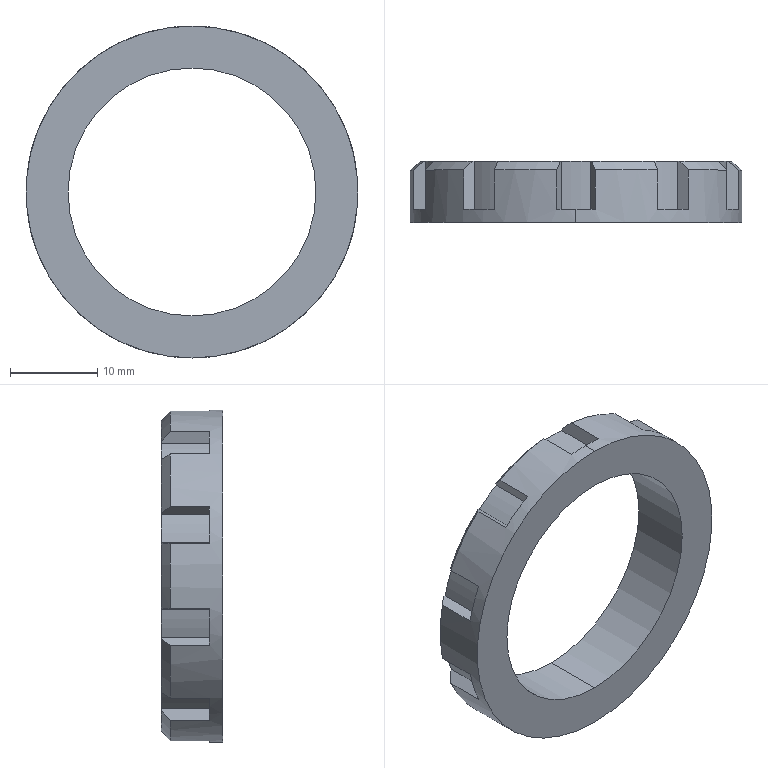Part | SolidWorks | features BaseBody 1 | 1 solid | 56 faces | box 38 x 7 x 38 mm | volume 3168 mm3 | plane 32 | cylinder 14 | cone 10 | commonest cylinder face diameters 35.2 x10 28.376 x2 38 x2